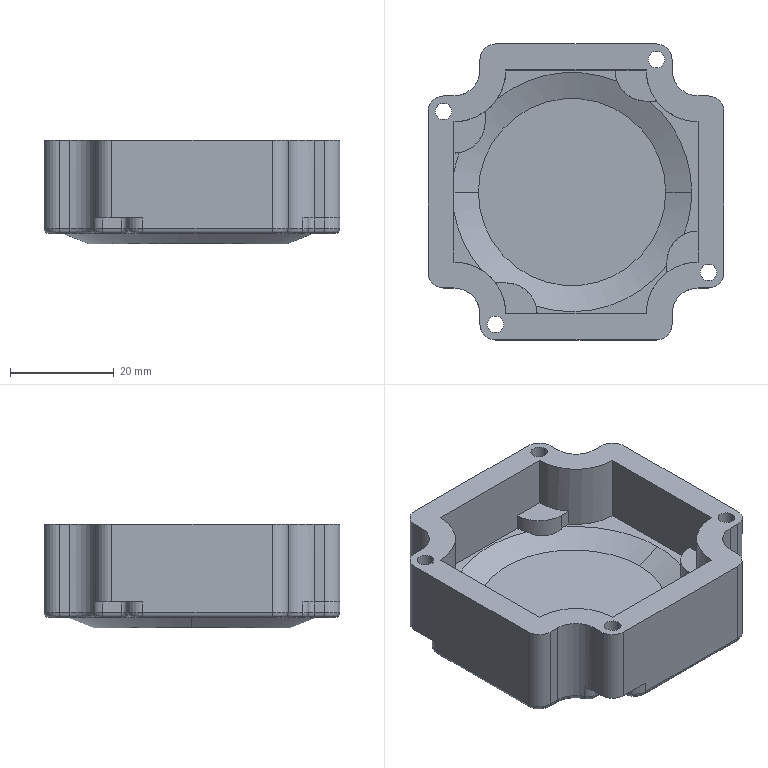Part | SolidWorks | features BaseBody 1 | 1 solid | 125 faces | box 57 x 57 x 20 mm | volume 26453 mm3 | cylinder 56 | plane 45 | torus 20 | cone 4 | commonest cylinder face diameters 2 x20 6 x12 3.2 x8 4 x4 10 x4 12 x4